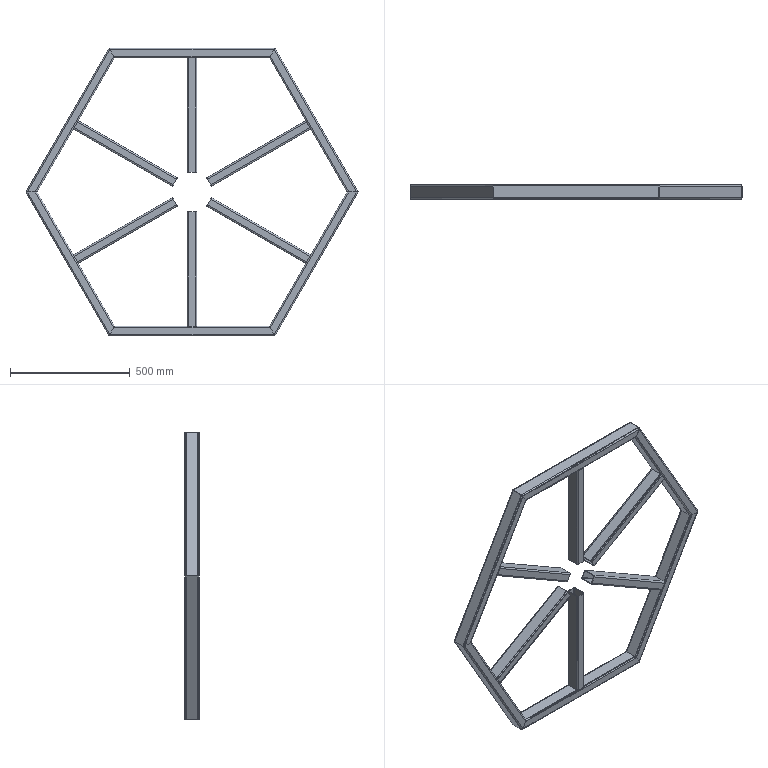Part | SolidWorks | features WeldCornerFeat 6, CirPattern 1, RefAxis 1, WeldMemberFeat 1, WeldmentFeature 1 | 12 solids | 216 faces | box 1386 x 60 x 1200 mm | volume 3722678 mm3 | plane 120 | cylinder 96 | commonest cylinder face diameters 6 x48 12 x48